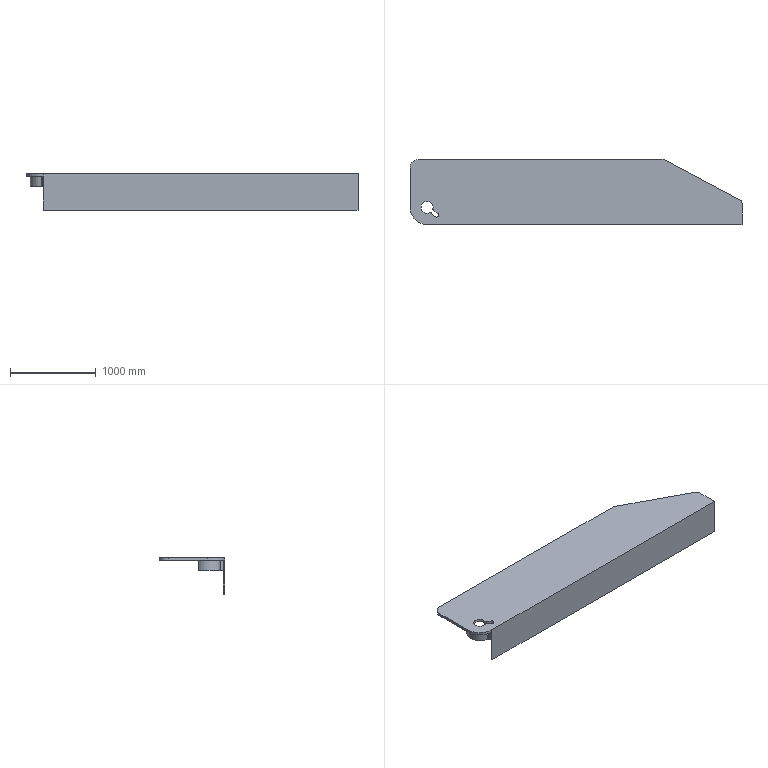Part | NX | features 顶梁侧护板左 2 | 1 solid | 51 faces | box 3880 x 760 x 430 mm | volume 99665785 mm3 | plane 35 | cylinder 16 | commonest cylinder face diameters 20 x6 40 x2 50 x1 100 x1 140 x1 160 x1